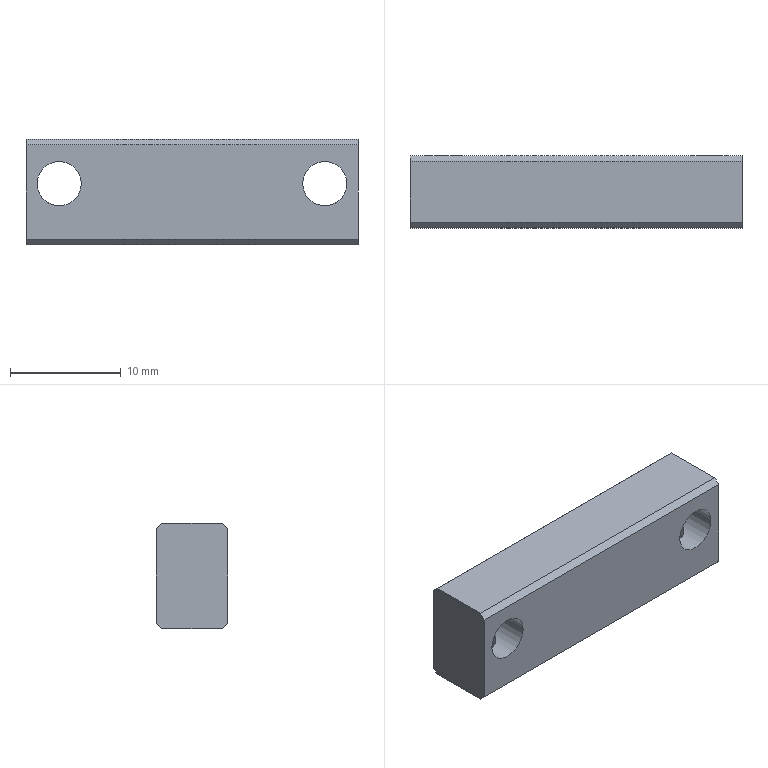Part | SolidWorks | features Chamfer 1, Extrusion 1, HoleWzd 1, ICE 1 | 1 solid | 18 faces | box 30 x 6.5 x 9.5 mm | volume 1639 mm3 | plane 10 | cylinder 8 | commonest cylinder face diameters 2.5 x4 4 x4
STEP:
#1=CARTESIAN_POINT('',(-10.75,0.,3.939));
#2=VERTEX_POINT('',#1);
#3=CARTESIAN_POINT('',(-13.25,0.,3.939));
#4=VERTEX_POINT('',#3);
#5=CARTESIAN_POINT('',(-10.75,0.,3.939));
#6=CARTESIAN_POINT('',(-10.75,-0.1694,3.939));
#7=CARTESIAN_POINT('',(-10.785,-0.3359,3.909));
#8=CARTESIAN_POINT('',(-10.911,-0.6351,3.821));
#9=CARTESIAN_POINT('',(-11.002,-0.7688,3.763));
#10=CARTESIAN_POINT('',(-11.227,-0.995,3.651));
#11=CARTESIAN_POINT('',(-11.359,-1.086,3.599));
#12=CARTESIAN_POINT('',(-11.664,-1.215,3.522));
#13=CARTESIAN_POINT('',(-11.829,-1.25,3.5));
#14=CARTESIAN_POINT('',(-12.167,-1.25,3.5));
#15=CARTESIAN_POINT('',(-12.335,-1.215,3.522));
#16=CARTESIAN_POINT('',(-12.637,-1.088,3.598));
#17=CARTESIAN_POINT('',(-12.772,-0.996,3.651));
#18=CARTESIAN_POINT('',(-12.997,-0.7702,3.762));
#19=CARTESIAN_POINT('',(-13.087,-0.6381,3.82));
#20=CARTESIAN_POINT('',(-13.215,-0.3367,3.909));
#21=CARTESIAN_POINT('',(-13.25,-0.1699,3.939));
#22=CARTESIAN_POINT('',(-13.25,0.,3.939));
#23=B_SPLINE_CURVE_WITH_KNOTS('',3,(#5,#6,#7,#8,#9,#10,#11,#12,#13,#14,#15,#16,#17,#18,#19,#20,#21,#22),.UNSPECIFIED.,.F.,.F.,(4,2,2,2,2,2,2,2,4),(0.004019,0.00452,0.005021,0.005522,0.006023,0.006524,0.007025,0.007526,0.008027),.UNSPECIFIED.);
#24=EDGE_CURVE('',#2,#4,#23,.T.);
#25=ORIENTED_EDGE('',*,*,#24,.F.);
#26=CARTESIAN_POINT('',(-10.75,0.,0.));
#27=VERTEX_POINT('',#26);
#28=CARTESIAN_POINT('',(-10.75,0.,0.));
#29=DIRECTION('',(0.,0.,-1.));
#30=VECTOR('',#29,1000.);
#31=LINE('',#28,#30);
#32=EDGE_CURVE('',#2,#27,#31,.T.);
#33=ORIENTED_EDGE('',*,*,#32,.T.);
#34=CARTESIAN_POINT('',(-13.25,0.,0.));
#35=VERTEX_POINT('',#34);
#36=CARTESIAN_POINT('',(-12.,0.,0.));
#37=DIRECTION('',(0.,0.,-1.));
#38=DIRECTION('',(-1.,0.,0.));
#39=AXIS2_PLACEMENT_3D('',#36,#37,#38);
#40=CIRCLE('',#39,1.25);
#41=EDGE_CURVE('',#27,#35,#40,.T.);
#42=ORIENTED_EDGE('',*,*,#41,.T.);
#43=CARTESIAN_POINT('',(-13.25,0.,0.));
#44=DIRECTION('',(0.,0.,-1.));
#45=VECTOR('',#44,1000.);
#46=LINE('',#43,#45);
#47=EDGE_CURVE('',#4,#35,#46,.T.);
#48=ORIENTED_EDGE('',*,*,#47,.F.);
#49=EDGE_LOOP('',(#25,#33,#42,#48));
#50=FACE_OUTER_BOUND('',#49,.T.);
#51=CARTESIAN_POINT('',(-12.,0.,0.));
#52=DIRECTION('',(0.,0.,-1.));
#53=DIRECTION('',(-1.,0.,0.));
#54=AXIS2_PLACEMENT_3D('',#51,#52,#53);
#55=CYLINDRICAL_SURFACE('',#54,1.25);
#56=ADVANCED_FACE('',(#50),#55,.F.);
#57=CARTESIAN_POINT('',(13.25,0.,3.939));
#58=VERTEX_POINT('',#57);
#59=CARTESIAN_POINT('',(10.75,0.,3.939));
#60=VERTEX_POINT('',#59);
#61=CARTESIAN_POINT('',(13.25,0.,3.939));
#62=CARTESIAN_POINT('',(13.25,-0.1694,3.939));
#63=CARTESIAN_POINT('',(13.215,-0.3359,3.909));
#64=CARTESIAN_POINT('',(13.089,-0.6351,3.821));
#65=CARTESIAN_POINT('',(12.998,-0.7688,3.763));
#66=CARTESIAN_POINT('',(12.773,-0.995,3.651));
#67=CARTESIAN_POINT('',(12.641,-1.086,3.599));
#68=CARTESIAN_POINT('',(12.336,-1.215,3.522));
#69=CARTESIAN_POINT('',(12.171,-1.25,3.5));
#70=CARTESIAN_POINT('',(11.833,-1.25,3.5));
#71=CARTESIAN_POINT('',(11.665,-1.215,3.522));
#72=CARTESIAN_POINT('',(11.363,-1.088,3.598));
#73=CARTESIAN_POINT('',(11.228,-0.996,3.651));
#74=CARTESIAN_POINT('',(11.003,-0.7702,3.762));
#75=CARTESIAN_POINT('',(10.913,-0.6381,3.82));
#76=CARTESIAN_POINT('',(10.785,-0.3367,3.909));
#77=CARTESIAN_POINT('',(10.75,-0.1699,3.939));
#78=CARTESIAN_POINT('',(10.75,0.,3.939));
#79=B_SPLINE_CURVE_WITH_KNOTS('',3,(#61,#62,#63,#64,#65,#66,#67,#68,#69,#70,#71,#72,#73,#74,#75,#76,#77,#78),.UNSPECIFIED.,.F.,.F.,(4,2,2,2,2,2,2,2,4),(0.004019,0.00452,0.005021,0.005522,0.006023,0.006524,0.007025,0.007526,0.008027),.UNSPECIFIED.);
#80=EDGE_CURVE('',#58,#60,#79,.T.);
#81=ORIENTED_EDGE('',*,*,#80,.F.);
#82=CARTESIAN_POINT('',(13.25,0.,0.));
#83=VERTEX_POINT('',#82);
#84=CARTESIAN_POINT('',(13.25,0.,0.));
#85=DIRECTION('',(0.,0.,-1.));
#86=VECTOR('',#85,1000.);
#87=LINE('',#84,#86);
#88=EDGE_CURVE('',#58,#83,#87,.T.);
#89=ORIENTED_EDGE('',*,*,#88,.T.);
#90=CARTESIAN_POINT('',(10.75,0.,0.));
#91=VERTEX_POINT('',#90);
#92=CARTESIAN_POINT('',(12.,0.,0.));
#93=DIRECTION('',(0.,0.,-1.));
#94=DIRECTION('',(-1.,0.,0.));
#95=AXIS2_PLACEMENT_3D('',#92,#93,#94);
#96=CIRCLE('',#95,1.25);
#97=EDGE_CURVE('',#83,#91,#96,.T.);
#98=ORIENTED_EDGE('',*,*,#97,.T.);
#99=CARTESIAN_POINT('',(10.75,0.,0.));
#100=DIRECTION('',(0.,0.,-1.));
#101=VECTOR('',#100,1000.);
#102=LINE('',#99,#101);
#103=EDGE_CURVE('',#60,#91,#102,.T.);
#104=ORIENTED_EDGE('',*,*,#103,.F.);
#105=EDGE_LOOP('',(#81,#89,#98,#104));
#106=FACE_OUTER_BOUND('',#105,.T.);
#107=CARTESIAN_POINT('',(12.,0.,0.));
#108=DIRECTION('',(0.,0.,-1.));
#109=DIRECTION('',(-1.,0.,0.));
#110=AXIS2_PLACEMENT_3D('',#107,#108,#109);
#111=CYLINDRICAL_SURFACE('',#110,1.25);
#112=ADVANCED_FACE('',(#106),#111,.F.);
#113=CARTESIAN_POINT('',(10.75,0.,3.939));
#114=CARTESIAN_POINT('',(10.75,0.0852,3.939));
#115=CARTESIAN_POINT('',(10.759,0.1683,3.932));
#116=CARTESIAN_POINT('',(10.792,0.3308,3.906));
#117=CARTESIAN_POINT('',(10.817,0.4107,3.887));
#118=CARTESIAN_POINT('',(10.911,0.6351,3.821));
#119=CARTESIAN_POINT('',(11.002,0.7693,3.762));
#120=CARTESIAN_POINT('',(11.226,0.9943,3.652));
#121=CARTESIAN_POINT('',(11.361,1.086,3.599));
#122=CARTESIAN_POINT('',(11.586,1.182,3.542));
#123=CARTESIAN_POINT('',(11.667,1.208,3.526));
#124=CARTESIAN_POINT('',(11.83,1.241,3.506));
#125=CARTESIAN_POINT('',(11.913,1.25,3.5));
#126=CARTESIAN_POINT('',(12.167,1.25,3.5));
#127=CARTESIAN_POINT('',(12.335,1.215,3.522));
#128=CARTESIAN_POINT('',(12.638,1.088,3.598));
#129=CARTESIAN_POINT('',(12.773,0.995,3.651));
#130=CARTESIAN_POINT('',(12.997,0.77,3.762));
#131=CARTESIAN_POINT('',(13.088,0.636,3.82));
#132=CARTESIAN_POINT('',(13.214,0.3378,3.909));
#133=CARTESIAN_POINT('',(13.25,0.1699,3.939));
#134=CARTESIAN_POINT('',(13.25,0.,3.939));
#135=B_SPLINE_CURVE_WITH_KNOTS('',3,(#113,#114,#115,#116,#117,#118,#119,#120,#121,#122,#123,#124,#125,#126,#127,#128,#129,#130,#131,#132,#133,#134),.UNSPECIFIED.,.F.,.F.,(4,2,2,2,2,2,2,2,2,2,4),(0.,0.0002512,0.0005023,0.001005,0.001507,0.001758,0.002009,0.002512,0.003014,0.003516,0.004019),.UNSPECIFIED.);
#136=EDGE_CURVE('',#60,#58,#135,.T.);
#137=ORIENTED_EDGE('',*,*,#136,.T.);
#138=ORIENTED_EDGE('',*,*,#80,.T.);
#139=EDGE_LOOP('',(#137,#138));
#140=FACE_BOUND('',#139,.T.);
#141=CARTESIAN_POINT('',(14.,-3.25,5.5));
#142=VERTEX_POINT('',#141);
#143=CARTESIAN_POINT('',(10.,-3.25,5.5));
#144=VERTEX_POINT('',#143);
#145=CARTESIAN_POINT('',(12.,-3.25,5.5));
#146=DIRECTION('',(0.,1.,0.));
#147=DIRECTION('',(-1.,0.,0.));
#148=AXIS2_PLACEMENT_3D('',#145,#146,#147);
#149=CIRCLE('',#148,2.);
#150=EDGE_CURVE('',#142,#144,#149,.T.);
#151=ORIENTED_EDGE('',*,*,#150,.F.);
#152=CARTESIAN_POINT('',(14.,3.25,5.5));
#153=VERTEX_POINT('',#152);
#154=CARTESIAN_POINT('',(14.,-3.25,5.5));
#155=DIRECTION('',(0.,1.,0.));
#156=VECTOR('',#155,1000.);
#157=LINE('',#154,#156);
#158=EDGE_CURVE('',#142,#153,#157,.T.);
#159=ORIENTED_EDGE('',*,*,#158,.T.);
#160=CARTESIAN_POINT('',(10.,3.25,5.5));
#161=VERTEX_POINT('',#160);
#162=CARTESIAN_POINT('',(12.,3.25,5.5));
#163=DIRECTION('',(0.,1.,0.));
#164=DIRECTION('',(-1.,0.,0.));
#165=AXIS2_PLACEMENT_3D('',#162,#163,#164);
#166=CIRCLE('',#165,2.);
#167=EDGE_CURVE('',#153,#161,#166,.T.);
#168=ORIENTED_EDGE('',*,*,#167,.T.);
#169=CARTESIAN_POINT('',(10.,-3.25,5.5));
#170=DIRECTION('',(0.,1.,0.));
#171=VECTOR('',#170,1000.);
#172=LINE('',#169,#171);
#173=EDGE_CURVE('',#144,#161,#172,.T.);
#174=ORIENTED_EDGE('',*,*,#173,.F.);
#175=EDGE_LOOP('',(#151,#159,#168,#174));
#176=FACE_OUTER_BOUND('',#175,.T.);
#177=CARTESIAN_POINT('',(12.,-3.25,5.5));
#178=DIRECTION('',(0.,1.,0.));
#179=DIRECTION('',(-1.,0.,0.));
#180=AXIS2_PLACEMENT_3D('',#177,#178,#179);
#181=CYLINDRICAL_SURFACE('',#180,2.);
#182=ADVANCED_FACE('',(#140,#176),#181,.F.);
#183=CARTESIAN_POINT('',(-13.25,0.,3.939));
#184=CARTESIAN_POINT('',(-13.25,0.0852,3.939));
#185=CARTESIAN_POINT('',(-13.241,0.1683,3.932));
#186=CARTESIAN_POINT('',(-13.208,0.3308,3.906));
#187=CARTESIAN_POINT('',(-13.183,0.4107,3.887));
#188=CARTESIAN_POINT('',(-13.089,0.6351,3.821));
#189=CARTESIAN_POINT('',(-12.998,0.7693,3.762));
#190=CARTESIAN_POINT('',(-12.774,0.9943,3.652));
#191=CARTESIAN_POINT('',(-12.639,1.086,3.599));
#192=CARTESIAN_POINT('',(-12.414,1.182,3.542));
#193=CARTESIAN_POINT('',(-12.333,1.208,3.526));
#194=CARTESIAN_POINT('',(-12.17,1.241,3.506));
#195=CARTESIAN_POINT('',(-12.087,1.25,3.5));
#196=CARTESIAN_POINT('',(-11.833,1.25,3.5));
#197=CARTESIAN_POINT('',(-11.665,1.215,3.522));
#198=CARTESIAN_POINT('',(-11.362,1.088,3.598));
#199=CARTESIAN_POINT('',(-11.227,0.995,3.651));
#200=CARTESIAN_POINT('',(-11.003,0.77,3.762));
#201=CARTESIAN_POINT('',(-10.912,0.636,3.82));
#202=CARTESIAN_POINT('',(-10.786,0.3378,3.909));
#203=CARTESIAN_POINT('',(-10.75,0.1699,3.939));
#204=CARTESIAN_POINT('',(-10.75,0.,3.939));
#205=B_SPLINE_CURVE_WITH_KNOTS('',3,(#183,#184,#185,#186,#187,#188,#189,#190,#191,#192,#193,#194,#195,#196,#197,#198,#199,#200,#201,#202,#203,#204),.UNSPECIFIED.,.F.,.F.,(4,2,2,2,2,2,2,2,2,2,4),(0.,0.0002512,0.0005023,0.001005,0.001507,0.001758,0.002009,0.002512,0.003014,0.003516,0.004019),.UNSPECIFIED.);
#206=EDGE_CURVE('',#4,#2,#205,.T.);
#207=ORIENTED_EDGE('',*,*,#206,.T.);
#208=ORIENTED_EDGE('',*,*,#24,.T.);
#209=EDGE_LOOP('',(#207,#208));
#210=FACE_BOUND('',#209,.T.);
#211=CARTESIAN_POINT('',(-10.,-3.25,5.5));
#212=VERTEX_POINT('',#211);
#213=CARTESIAN_POINT('',(-14.,-3.25,5.5));
#214=VERTEX_POINT('',#213);
#215=CARTESIAN_POINT('',(-12.,-3.25,5.5));
#216=DIRECTION('',(0.,1.,0.));
#217=DIRECTION('',(-1.,0.,0.));
#218=AXIS2_PLACEMENT_3D('',#215,#216,#217);
#219=CIRCLE('',#218,2.);
#220=EDGE_CURVE('',#212,#214,#219,.T.);
#221=ORIENTED_EDGE('',*,*,#220,.F.);
#222=CARTESIAN_POINT('',(-10.,3.25,5.5));
#223=VERTEX_POINT('',#222);
#224=CARTESIAN_POINT('',(-10.,-3.25,5.5));
#225=DIRECTION('',(0.,1.,0.));
#226=VECTOR('',#225,1000.);
#227=LINE('',#224,#226);
#228=EDGE_CURVE('',#212,#223,#227,.T.);
#229=ORIENTED_EDGE('',*,*,#228,.T.);
#230=CARTESIAN_POINT('',(-14.,3.25,5.5));
#231=VERTEX_POINT('',#230);
#232=CARTESIAN_POINT('',(-12.,3.25,5.5));
#233=DIRECTION('',(0.,1.,0.));
#234=DIRECTION('',(-1.,0.,0.));
#235=AXIS2_PLACEMENT_3D('',#232,#233,#234);
#236=CIRCLE('',#235,2.);
#237=EDGE_CURVE('',#223,#231,#236,.T.);
#238=ORIENTED_EDGE('',*,*,#237,.T.);
#239=CARTESIAN_POINT('',(-14.,-3.25,5.5));
#240=DIRECTION('',(0.,1.,0.));
#241=VECTOR('',#240,1000.);
#242=LINE('',#239,#241);
#243=EDGE_CURVE('',#214,#231,#242,.T.);
#244=ORIENTED_EDGE('',*,*,#243,.F.);
#245=EDGE_LOOP('',(#221,#229,#238,#244));
#246=FACE_OUTER_BOUND('',#245,.T.);
#247=CARTESIAN_POINT('',(-12.,-3.25,5.5));
#248=DIRECTION('',(0.,1.,0.));
#249=DIRECTION('',(-1.,0.,0.));
#250=AXIS2_PLACEMENT_3D('',#247,#248,#249);
#251=CYLINDRICAL_SURFACE('',#250,2.);
#252=ADVANCED_FACE('',(#210,#246),#251,.F.);
#253=CARTESIAN_POINT('',(-15.,3.25,9.));
#254=VERTEX_POINT('',#253);
#255=CARTESIAN_POINT('',(-15.,3.25,0.5));
#256=VERTEX_POINT('',#255);
#257=CARTESIAN_POINT('',(-15.,3.25,9.5));
#258=DIRECTION('',(0.,0.,-1.));
#259=VECTOR('',#258,1000.);
#260=LINE('',#257,#259);
#261=EDGE_CURVE('',#254,#256,#260,.T.);
#262=ORIENTED_EDGE('',*,*,#261,.T.);
#263=CARTESIAN_POINT('',(-15.,2.75,0.));
#264=VERTEX_POINT('',#263);
#265=CARTESIAN_POINT('',(-15.,3.25,0.5));
#266=DIRECTION('',(0.,-0.7071,-0.7071));
#267=VECTOR('',#266,1000.);
#268=LINE('',#265,#267);
#269=EDGE_CURVE('',#256,#264,#268,.T.);
#270=ORIENTED_EDGE('',*,*,#269,.T.);
#271=CARTESIAN_POINT('',(-15.,-2.75,0.));
#272=VERTEX_POINT('',#271);
#273=CARTESIAN_POINT('',(-15.,-3.25,0.));
#274=DIRECTION('',(0.,-1.,0.));
#275=VECTOR('',#274,1000.);
#276=LINE('',#273,#275);
#277=EDGE_CURVE('',#264,#272,#276,.T.);
#278=ORIENTED_EDGE('',*,*,#277,.T.);
#279=CARTESIAN_POINT('',(-15.,-3.25,0.5));
#280=VERTEX_POINT('',#279);
#281=CARTESIAN_POINT('',(-15.,-3.25,0.5));
#282=DIRECTION('',(0.,-0.7071,0.7071));
#283=VECTOR('',#282,1000.);
#284=LINE('',#281,#283);
#285=EDGE_CURVE('',#272,#280,#284,.T.);
#286=ORIENTED_EDGE('',*,*,#285,.T.);
#287=CARTESIAN_POINT('',(-15.,-3.25,9.));
#288=VERTEX_POINT('',#287);
#289=CARTESIAN_POINT('',(-15.,-3.25,9.5));
#290=DIRECTION('',(0.,0.,-1.));
#291=VECTOR('',#290,1000.);
#292=LINE('',#289,#291);
#293=EDGE_CURVE('',#288,#280,#292,.T.);
#294=ORIENTED_EDGE('',*,*,#293,.F.);
#295=CARTESIAN_POINT('',(-15.,-2.75,9.5));
#296=VERTEX_POINT('',#295);
#297=CARTESIAN_POINT('',(-15.,-2.75,9.5));
#298=DIRECTION('',(0.,0.7071,0.7071));
#299=VECTOR('',#298,1000.);
#300=LINE('',#297,#299);
#301=EDGE_CURVE('',#288,#296,#300,.T.);
#302=ORIENTED_EDGE('',*,*,#301,.T.);
#303=CARTESIAN_POINT('',(-15.,2.75,9.5));
#304=VERTEX_POINT('',#303);
#305=CARTESIAN_POINT('',(-15.,-3.25,9.5));
#306=DIRECTION('',(0.,-1.,0.));
#307=VECTOR('',#306,1000.);
#308=LINE('',#305,#307);
#309=EDGE_CURVE('',#304,#296,#308,.T.);
#310=ORIENTED_EDGE('',*,*,#309,.F.);
#311=CARTESIAN_POINT('',(-15.,2.75,9.5));
#312=DIRECTION('',(0.,0.7071,-0.7071));
#313=VECTOR('',#312,1000.);
#314=LINE('',#311,#313);
#315=EDGE_CURVE('',#304,#254,#314,.T.);
#316=ORIENTED_EDGE('',*,*,#315,.T.);
#317=EDGE_LOOP('',(#262,#270,#278,#286,#294,#302,#310,#316));
#318=FACE_OUTER_BOUND('',#317,.T.);
#319=CARTESIAN_POINT('',(-15.,-3.25,9.5));
#320=DIRECTION('',(1.,0.,0.));
#321=DIRECTION('',(0.,0.,-1.));
#322=AXIS2_PLACEMENT_3D('',#319,#320,#321);
#323=PLANE('',#322);
#324=ADVANCED_FACE('',(#318),#323,.F.);
#325=CARTESIAN_POINT('',(12.,-3.25,5.5));
#326=DIRECTION('',(0.,1.,0.));
#327=DIRECTION('',(-1.,0.,0.));
#328=AXIS2_PLACEMENT_3D('',#325,#326,#327);
#329=CIRCLE('',#328,2.);
#330=EDGE_CURVE('',#144,#142,#329,.T.);
#331=ORIENTED_EDGE('',*,*,#330,.T.);
#332=ORIENTED_EDGE('',*,*,#150,.T.);
#333=EDGE_LOOP('',(#331,#332));
#334=FACE_BOUND('',#333,.T.);
#335=CARTESIAN_POINT('',(-12.,-3.25,5.5));
#336=DIRECTION('',(0.,1.,0.));
#337=DIRECTION('',(-1.,0.,0.));
#338=AXIS2_PLACEMENT_3D('',#335,#336,#337);
#339=CIRCLE('',#338,2.);
#340=EDGE_CURVE('',#214,#212,#339,.T.);
#341=ORIENTED_EDGE('',*,*,#340,.T.);
#342=ORIENTED_EDGE('',*,*,#220,.T.);
#343=EDGE_LOOP('',(#341,#342));
#344=FACE_BOUND('',#343,.T.);
#345=CARTESIAN_POINT('',(15.,-3.25,9.));
#346=VERTEX_POINT('',#345);
#347=CARTESIAN_POINT('',(15.,-3.25,0.5));
#348=VERTEX_POINT('',#347);
#349=CARTESIAN_POINT('',(15.,-3.25,9.5));
#350=DIRECTION('',(0.,0.,-1.));
#351=VECTOR('',#350,1000.);
#352=LINE('',#349,#351);
#353=EDGE_CURVE('',#346,#348,#352,.T.);
#354=ORIENTED_EDGE('',*,*,#353,.F.);
#355=CARTESIAN_POINT('',(-15.,-3.25,9.));
#356=DIRECTION('',(-1.,0.,0.));
#357=VECTOR('',#356,1000.);
#358=LINE('',#355,#357);
#359=EDGE_CURVE('',#346,#288,#358,.T.);
#360=ORIENTED_EDGE('',*,*,#359,.T.);
#361=ORIENTED_EDGE('',*,*,#293,.T.);
#362=CARTESIAN_POINT('',(15.,-3.25,0.5));
#363=DIRECTION('',(1.,0.,0.));
#364=VECTOR('',#363,1000.);
#365=LINE('',#362,#364);
#366=EDGE_CURVE('',#280,#348,#365,.T.);
#367=ORIENTED_EDGE('',*,*,#366,.T.);
#368=EDGE_LOOP('',(#354,#360,#361,#367));
#369=FACE_OUTER_BOUND('',#368,.T.);
#370=CARTESIAN_POINT('',(15.,-3.25,9.5));
#371=DIRECTION('',(0.,1.,0.));
#372=DIRECTION('',(-1.,0.,0.));
#373=AXIS2_PLACEMENT_3D('',#370,#371,#372);
#374=PLANE('',#373);
#375=ADVANCED_FACE('',(#334,#344,#369),#374,.F.);
#376=CARTESIAN_POINT('',(15.,-2.75,0.));
#377=VERTEX_POINT('',#376);
#378=CARTESIAN_POINT('',(15.,2.75,0.));
#379=VERTEX_POINT('',#378);
#380=CARTESIAN_POINT('',(15.,-3.25,0.));
#381=DIRECTION('',(0.,1.,0.));
#382=VECTOR('',#381,1000.);
#383=LINE('',#380,#382);
#384=EDGE_CURVE('',#377,#379,#383,.T.);
#385=ORIENTED_EDGE('',*,*,#384,.T.);
#386=CARTESIAN_POINT('',(15.,3.25,0.5));
#387=VERTEX_POINT('',#386);
#388=CARTESIAN_POINT('',(15.,3.25,0.5));
#389=DIRECTION('',(0.,0.7071,0.7071));
#390=VECTOR('',#389,1000.);
#391=LINE('',#388,#390);
#392=EDGE_CURVE('',#379,#387,#391,.T.);
#393=ORIENTED_EDGE('',*,*,#392,.T.);
#394=CARTESIAN_POINT('',(15.,3.25,9.));
#395=VERTEX_POINT('',#394);
#396=CARTESIAN_POINT('',(15.,3.25,9.5));
#397=DIRECTION('',(0.,0.,-1.));
#398=VECTOR('',#397,1000.);
#399=LINE('',#396,#398);
#400=EDGE_CURVE('',#395,#387,#399,.T.);
#401=ORIENTED_EDGE('',*,*,#400,.F.);
#402=CARTESIAN_POINT('',(15.,2.75,9.5));
#403=VERTEX_POINT('',#402);
#404=CARTESIAN_POINT('',(15.,2.75,9.5));
#405=DIRECTION('',(0.,-0.7071,0.7071));
#406=VECTOR('',#405,1000.);
#407=LINE('',#404,#406);
#408=EDGE_CURVE('',#395,#403,#407,.T.);
#409=ORIENTED_EDGE('',*,*,#408,.T.);
#410=CARTESIAN_POINT('',(15.,-2.75,9.5));
#411=VERTEX_POINT('',#410);
#412=CARTESIAN_POINT('',(15.,-3.25,9.5));
#413=DIRECTION('',(0.,1.,0.));
#414=VECTOR('',#413,1000.);
#415=LINE('',#412,#414);
#416=EDGE_CURVE('',#411,#403,#415,.T.);
#417=ORIENTED_EDGE('',*,*,#416,.F.);
#418=CARTESIAN_POINT('',(15.,-2.75,9.5));
#419=DIRECTION('',(0.,-0.7071,-0.7071));
#420=VECTOR('',#419,1000.);
#421=LINE('',#418,#420);
#422=EDGE_CURVE('',#411,#346,#421,.T.);
#423=ORIENTED_EDGE('',*,*,#422,.T.);
#424=ORIENTED_EDGE('',*,*,#353,.T.);
#425=CARTESIAN_POINT('',(15.,-3.25,0.5));
#426=DIRECTION('',(0.,0.7071,-0.7071));
#427=VECTOR('',#426,1000.);
#428=LINE('',#425,#427);
#429=EDGE_CURVE('',#348,#377,#428,.T.);
#430=ORIENTED_EDGE('',*,*,#429,.T.);
#431=EDGE_LOOP('',(#385,#393,#401,#409,#417,#423,#424,#430));
#432=FACE_OUTER_BOUND('',#431,.T.);
#433=CARTESIAN_POINT('',(15.,-3.25,9.5));
#434=DIRECTION('',(-1.,0.,0.));
#435=DIRECTION('',(0.,0.,1.));
#436=AXIS2_PLACEMENT_3D('',#433,#434,#435);
#437=PLANE('',#436);
#438=ADVANCED_FACE('',(#432),#437,.F.);
#439=CARTESIAN_POINT('',(12.,3.25,5.5));
#440=DIRECTION('',(0.,1.,0.));
#441=DIRECTION('',(-1.,0.,0.));
#442=AXIS2_PLACEMENT_3D('',#439,#440,#441);
#443=CIRCLE('',#442,2.);
#444=EDGE_CURVE('',#161,#153,#443,.T.);
#445=ORIENTED_EDGE('',*,*,#444,.F.);
#446=ORIENTED_EDGE('',*,*,#167,.F.);
#447=EDGE_LOOP('',(#445,#446));
#448=FACE_BOUND('',#447,.T.);
#449=CARTESIAN_POINT('',(-12.,3.25,5.5));
#450=DIRECTION('',(0.,1.,0.));
#451=DIRECTION('',(-1.,0.,0.));
#452=AXIS2_PLACEMENT_3D('',#449,#450,#451);
#453=CIRCLE('',#452,2.);
#454=EDGE_CURVE('',#231,#223,#453,.T.);
#455=ORIENTED_EDGE('',*,*,#454,.F.);
#456=ORIENTED_EDGE('',*,*,#237,.F.);
#457=EDGE_LOOP('',(#455,#456));
#458=FACE_BOUND('',#457,.T.);
#459=ORIENTED_EDGE('',*,*,#400,.T.);
#460=CARTESIAN_POINT('',(15.,3.25,0.5));
#461=DIRECTION('',(-1.,0.,0.));
#462=VECTOR('',#461,1000.);
#463=LINE('',#460,#462);
#464=EDGE_CURVE('',#387,#256,#463,.T.);
#465=ORIENTED_EDGE('',*,*,#464,.T.);
#466=ORIENTED_EDGE('',*,*,#261,.F.);
#467=CARTESIAN_POINT('',(15.,3.25,9.));
#468=DIRECTION('',(1.,0.,0.));
#469=VECTOR('',#468,1000.);
#470=LINE('',#467,#469);
#471=EDGE_CURVE('',#254,#395,#470,.T.);
#472=ORIENTED_EDGE('',*,*,#471,.T.);
#473=EDGE_LOOP('',(#459,#465,#466,#472));
#474=FACE_OUTER_BOUND('',#473,.T.);
#475=CARTESIAN_POINT('',(15.,3.25,9.5));
#476=DIRECTION('',(0.,-1.,0.));
#477=DIRECTION('',(1.,0.,0.));
#478=AXIS2_PLACEMENT_3D('',#475,#476,#477);
#479=PLANE('',#478);
#480=ADVANCED_FACE('',(#448,#458,#474),#479,.F.);
#481=ORIENTED_EDGE('',*,*,#416,.T.);
#482=CARTESIAN_POINT('',(-15.,2.75,9.5));
#483=DIRECTION('',(-1.,0.,0.));
#484=VECTOR('',#483,1000.);
#485=LINE('',#482,#484);
#486=EDGE_CURVE('',#403,#304,#485,.T.);
#487=ORIENTED_EDGE('',*,*,#486,.T.);
#488=ORIENTED_EDGE('',*,*,#309,.T.);
#489=CARTESIAN_POINT('',(15.,-2.75,9.5));
#490=DIRECTION('',(1.,0.,0.));
#491=VECTOR('',#490,1000.);
#492=LINE('',#489,#491);
#493=EDGE_CURVE('',#296,#411,#492,.T.);
#494=ORIENTED_EDGE('',*,*,#493,.T.);
#495=EDGE_LOOP('',(#481,#487,#488,#494));
#496=FACE_OUTER_BOUND('',#495,.T.);
#497=CARTESIAN_POINT('',(-15.,3.25,9.5));
#498=DIRECTION('',(0.,0.,1.));
#499=DIRECTION('',(1.,0.,0.));
#500=AXIS2_PLACEMENT_3D('',#497,#498,#499);
#501=PLANE('',#500);
#502=ADVANCED_FACE('',(#496),#501,.T.);
#503=CARTESIAN_POINT('',(-12.,0.,0.));
#504=DIRECTION('',(0.,0.,-1.));
#505=DIRECTION('',(-1.,0.,0.));
#506=AXIS2_PLACEMENT_3D('',#503,#504,#505);
#507=CIRCLE('',#506,1.25);
#508=EDGE_CURVE('',#35,#27,#507,.T.);
#509=ORIENTED_EDGE('',*,*,#508,.F.);
#510=ORIENTED_EDGE('',*,*,#41,.F.);
#511=EDGE_LOOP('',(#509,#510));
#512=FACE_BOUND('',#511,.T.);
#513=CARTESIAN_POINT('',(12.,0.,0.));
#514=DIRECTION('',(0.,0.,-1.));
#515=DIRECTION('',(-1.,0.,0.));
#516=AXIS2_PLACEMENT_3D('',#513,#514,#515);
#517=CIRCLE('',#516,1.25);
#518=EDGE_CURVE('',#91,#83,#517,.T.);
#519=ORIENTED_EDGE('',*,*,#518,.F.);
#520=ORIENTED_EDGE('',*,*,#97,.F.);
#521=EDGE_LOOP('',(#519,#520));
#522=FACE_BOUND('',#521,.T.);
#523=ORIENTED_EDGE('',*,*,#277,.F.);
#524=CARTESIAN_POINT('',(-15.,2.75,0.));
#525=DIRECTION('',(1.,0.,0.));
#526=VECTOR('',#525,1000.);
#527=LINE('',#524,#526);
#528=EDGE_CURVE('',#264,#379,#527,.T.);
#529=ORIENTED_EDGE('',*,*,#528,.T.);
#530=ORIENTED_EDGE('',*,*,#384,.F.);
#531=CARTESIAN_POINT('',(-15.,-2.75,0.));
#532=DIRECTION('',(-1.,0.,0.));
#533=VECTOR('',#532,1000.);
#534=LINE('',#531,#533);
#535=EDGE_CURVE('',#377,#272,#534,.T.);
#536=ORIENTED_EDGE('',*,*,#535,.T.);
#537=EDGE_LOOP('',(#523,#529,#530,#536));
#538=FACE_OUTER_BOUND('',#537,.T.);
#539=CARTESIAN_POINT('',(-15.,3.25,0.));
#540=DIRECTION('',(0.,0.,1.));
#541=DIRECTION('',(1.,0.,0.));
#542=AXIS2_PLACEMENT_3D('',#539,#540,#541);
#543=PLANE('',#542);
#544=ADVANCED_FACE('',(#512,#522,#538),#543,.F.);
#545=ORIENTED_EDGE('',*,*,#228,.F.);
#546=ORIENTED_EDGE('',*,*,#340,.F.);
#547=ORIENTED_EDGE('',*,*,#243,.T.);
#548=ORIENTED_EDGE('',*,*,#454,.T.);
#549=EDGE_LOOP('',(#545,#546,#547,#548));
#550=FACE_OUTER_BOUND('',#549,.T.);
#551=CARTESIAN_POINT('',(-12.,-3.25,5.5));
#552=DIRECTION('',(0.,1.,0.));
#553=DIRECTION('',(-1.,0.,0.));
#554=AXIS2_PLACEMENT_3D('',#551,#552,#553);
#555=CYLINDRICAL_SURFACE('',#554,2.);
#556=ADVANCED_FACE('',(#550),#555,.F.);
#557=ORIENTED_EDGE('',*,*,#158,.F.);
#558=ORIENTED_EDGE('',*,*,#330,.F.);
#559=ORIENTED_EDGE('',*,*,#173,.T.);
#560=ORIENTED_EDGE('',*,*,#444,.T.);
#561=EDGE_LOOP('',(#557,#558,#559,#560));
#562=FACE_OUTER_BOUND('',#561,.T.);
#563=CARTESIAN_POINT('',(12.,-3.25,5.5));
#564=DIRECTION('',(0.,1.,0.));
#565=DIRECTION('',(-1.,0.,0.));
#566=AXIS2_PLACEMENT_3D('',#563,#564,#565);
#567=CYLINDRICAL_SURFACE('',#566,2.);
#568=ADVANCED_FACE('',(#562),#567,.F.);
#569=ORIENTED_EDGE('',*,*,#88,.F.);
#570=ORIENTED_EDGE('',*,*,#136,.F.);
#571=ORIENTED_EDGE('',*,*,#103,.T.);
#572=ORIENTED_EDGE('',*,*,#518,.T.);
#573=EDGE_LOOP('',(#569,#570,#571,#572));
#574=FACE_OUTER_BOUND('',#573,.T.);
#575=CARTESIAN_POINT('',(12.,0.,0.));
#576=DIRECTION('',(0.,0.,-1.));
#577=DIRECTION('',(-1.,0.,0.));
#578=AXIS2_PLACEMENT_3D('',#575,#576,#577);
#579=CYLINDRICAL_SURFACE('',#578,1.25);
#580=ADVANCED_FACE('',(#574),#579,.F.);
#581=ORIENTED_EDGE('',*,*,#32,.F.);
#582=ORIENTED_EDGE('',*,*,#206,.F.);
#583=ORIENTED_EDGE('',*,*,#47,.T.);
#584=ORIENTED_EDGE('',*,*,#508,.T.);
#585=EDGE_LOOP('',(#581,#582,#583,#584));
#586=FACE_OUTER_BOUND('',#585,.T.);
#587=CARTESIAN_POINT('',(-12.,0.,0.));
#588=DIRECTION('',(0.,0.,-1.));
#589=DIRECTION('',(-1.,0.,0.));
#590=AXIS2_PLACEMENT_3D('',#587,#588,#589);
#591=CYLINDRICAL_SURFACE('',#590,1.25);
#592=ADVANCED_FACE('',(#586),#591,.F.);
#593=ORIENTED_EDGE('',*,*,#392,.F.);
#594=ORIENTED_EDGE('',*,*,#528,.F.);
#595=ORIENTED_EDGE('',*,*,#269,.F.);
#596=ORIENTED_EDGE('',*,*,#464,.F.);
#597=EDGE_LOOP('',(#593,#594,#595,#596));
#598=FACE_OUTER_BOUND('',#597,.T.);
#599=CARTESIAN_POINT('',(15.,3.25,0.5));
#600=DIRECTION('',(0.,-0.7071,0.7071));
#601=DIRECTION('',(-1.,0.,0.));
#602=AXIS2_PLACEMENT_3D('',#599,#600,#601);
#603=PLANE('',#602);
#604=ADVANCED_FACE('',(#598),#603,.F.);
#605=ORIENTED_EDGE('',*,*,#408,.F.);
#606=ORIENTED_EDGE('',*,*,#471,.F.);
#607=ORIENTED_EDGE('',*,*,#315,.F.);
#608=ORIENTED_EDGE('',*,*,#486,.F.);
#609=EDGE_LOOP('',(#605,#606,#607,#608));
#610=FACE_OUTER_BOUND('',#609,.T.);
#611=CARTESIAN_POINT('',(-15.,2.75,9.5));
#612=DIRECTION('',(0.,0.7071,0.7071));
#613=DIRECTION('',(1.,0.,0.));
#614=AXIS2_PLACEMENT_3D('',#611,#612,#613);
#615=PLANE('',#614);
#616=ADVANCED_FACE('',(#610),#615,.T.);
#617=ORIENTED_EDGE('',*,*,#301,.F.);
#618=ORIENTED_EDGE('',*,*,#359,.F.);
#619=ORIENTED_EDGE('',*,*,#422,.F.);
#620=ORIENTED_EDGE('',*,*,#493,.F.);
#621=EDGE_LOOP('',(#617,#618,#619,#620));
#622=FACE_OUTER_BOUND('',#621,.T.);
#623=CARTESIAN_POINT('',(-15.,-2.75,9.5));
#624=DIRECTION('',(0.,-0.7071,0.7071));
#625=DIRECTION('',(-1.,0.,0.));
#626=AXIS2_PLACEMENT_3D('',#623,#624,#625);
#627=PLANE('',#626);
#628=ADVANCED_FACE('',(#622),#627,.T.);
#629=ORIENTED_EDGE('',*,*,#285,.F.);
#630=ORIENTED_EDGE('',*,*,#535,.F.);
#631=ORIENTED_EDGE('',*,*,#429,.F.);
#632=ORIENTED_EDGE('',*,*,#366,.F.);
#633=EDGE_LOOP('',(#629,#630,#631,#632));
#634=FACE_OUTER_BOUND('',#633,.T.);
#635=CARTESIAN_POINT('',(15.,-3.25,0.5));
#636=DIRECTION('',(0.,0.7071,0.7071));
#637=DIRECTION('',(1.,0.,0.));
#638=AXIS2_PLACEMENT_3D('',#635,#636,#637);
#639=PLANE('',#638);
#640=ADVANCED_FACE('',(#634),#639,.F.);
#641=CLOSED_SHELL('',(#56,#112,#182,#252,#324,#375,#438,#480,#502,#544,#556,#568,#580,#592,#604,#616,#628,#640));
#642=MANIFOLD_SOLID_BREP('',#641);
#643=CARTESIAN_POINT('',(0.,0.,0.));
#644=DIRECTION('',(0.,0.,1.));
#645=DIRECTION('',(1.,0.,0.));
#646=AXIS2_PLACEMENT_3D('',#643,#644,#645);
#647=(LENGTH_UNIT()NAMED_UNIT(*)SI_UNIT(.MILLI.,.METRE.));
#648=UNCERTAINTY_MEASURE_WITH_UNIT(LENGTH_MEASURE(0.00001),#647,'','');
#649=(NAMED_UNIT(*)PLANE_ANGLE_UNIT()SI_UNIT($,.RADIAN.));
#650=(NAMED_UNIT(*)SI_UNIT($,.STERADIAN.)SOLID_ANGLE_UNIT());
#651=(GEOMETRIC_REPRESENTATION_CONTEXT(3)GLOBAL_UNCERTAINTY_ASSIGNED_CONTEXT((#648))GLOBAL_UNIT_ASSIGNED_CONTEXT((#647,#649,#650))REPRESENTATION_CONTEXT('',''));
#652=ADVANCED_BREP_SHAPE_REPRESENTATION('',(#642,#646),#651);